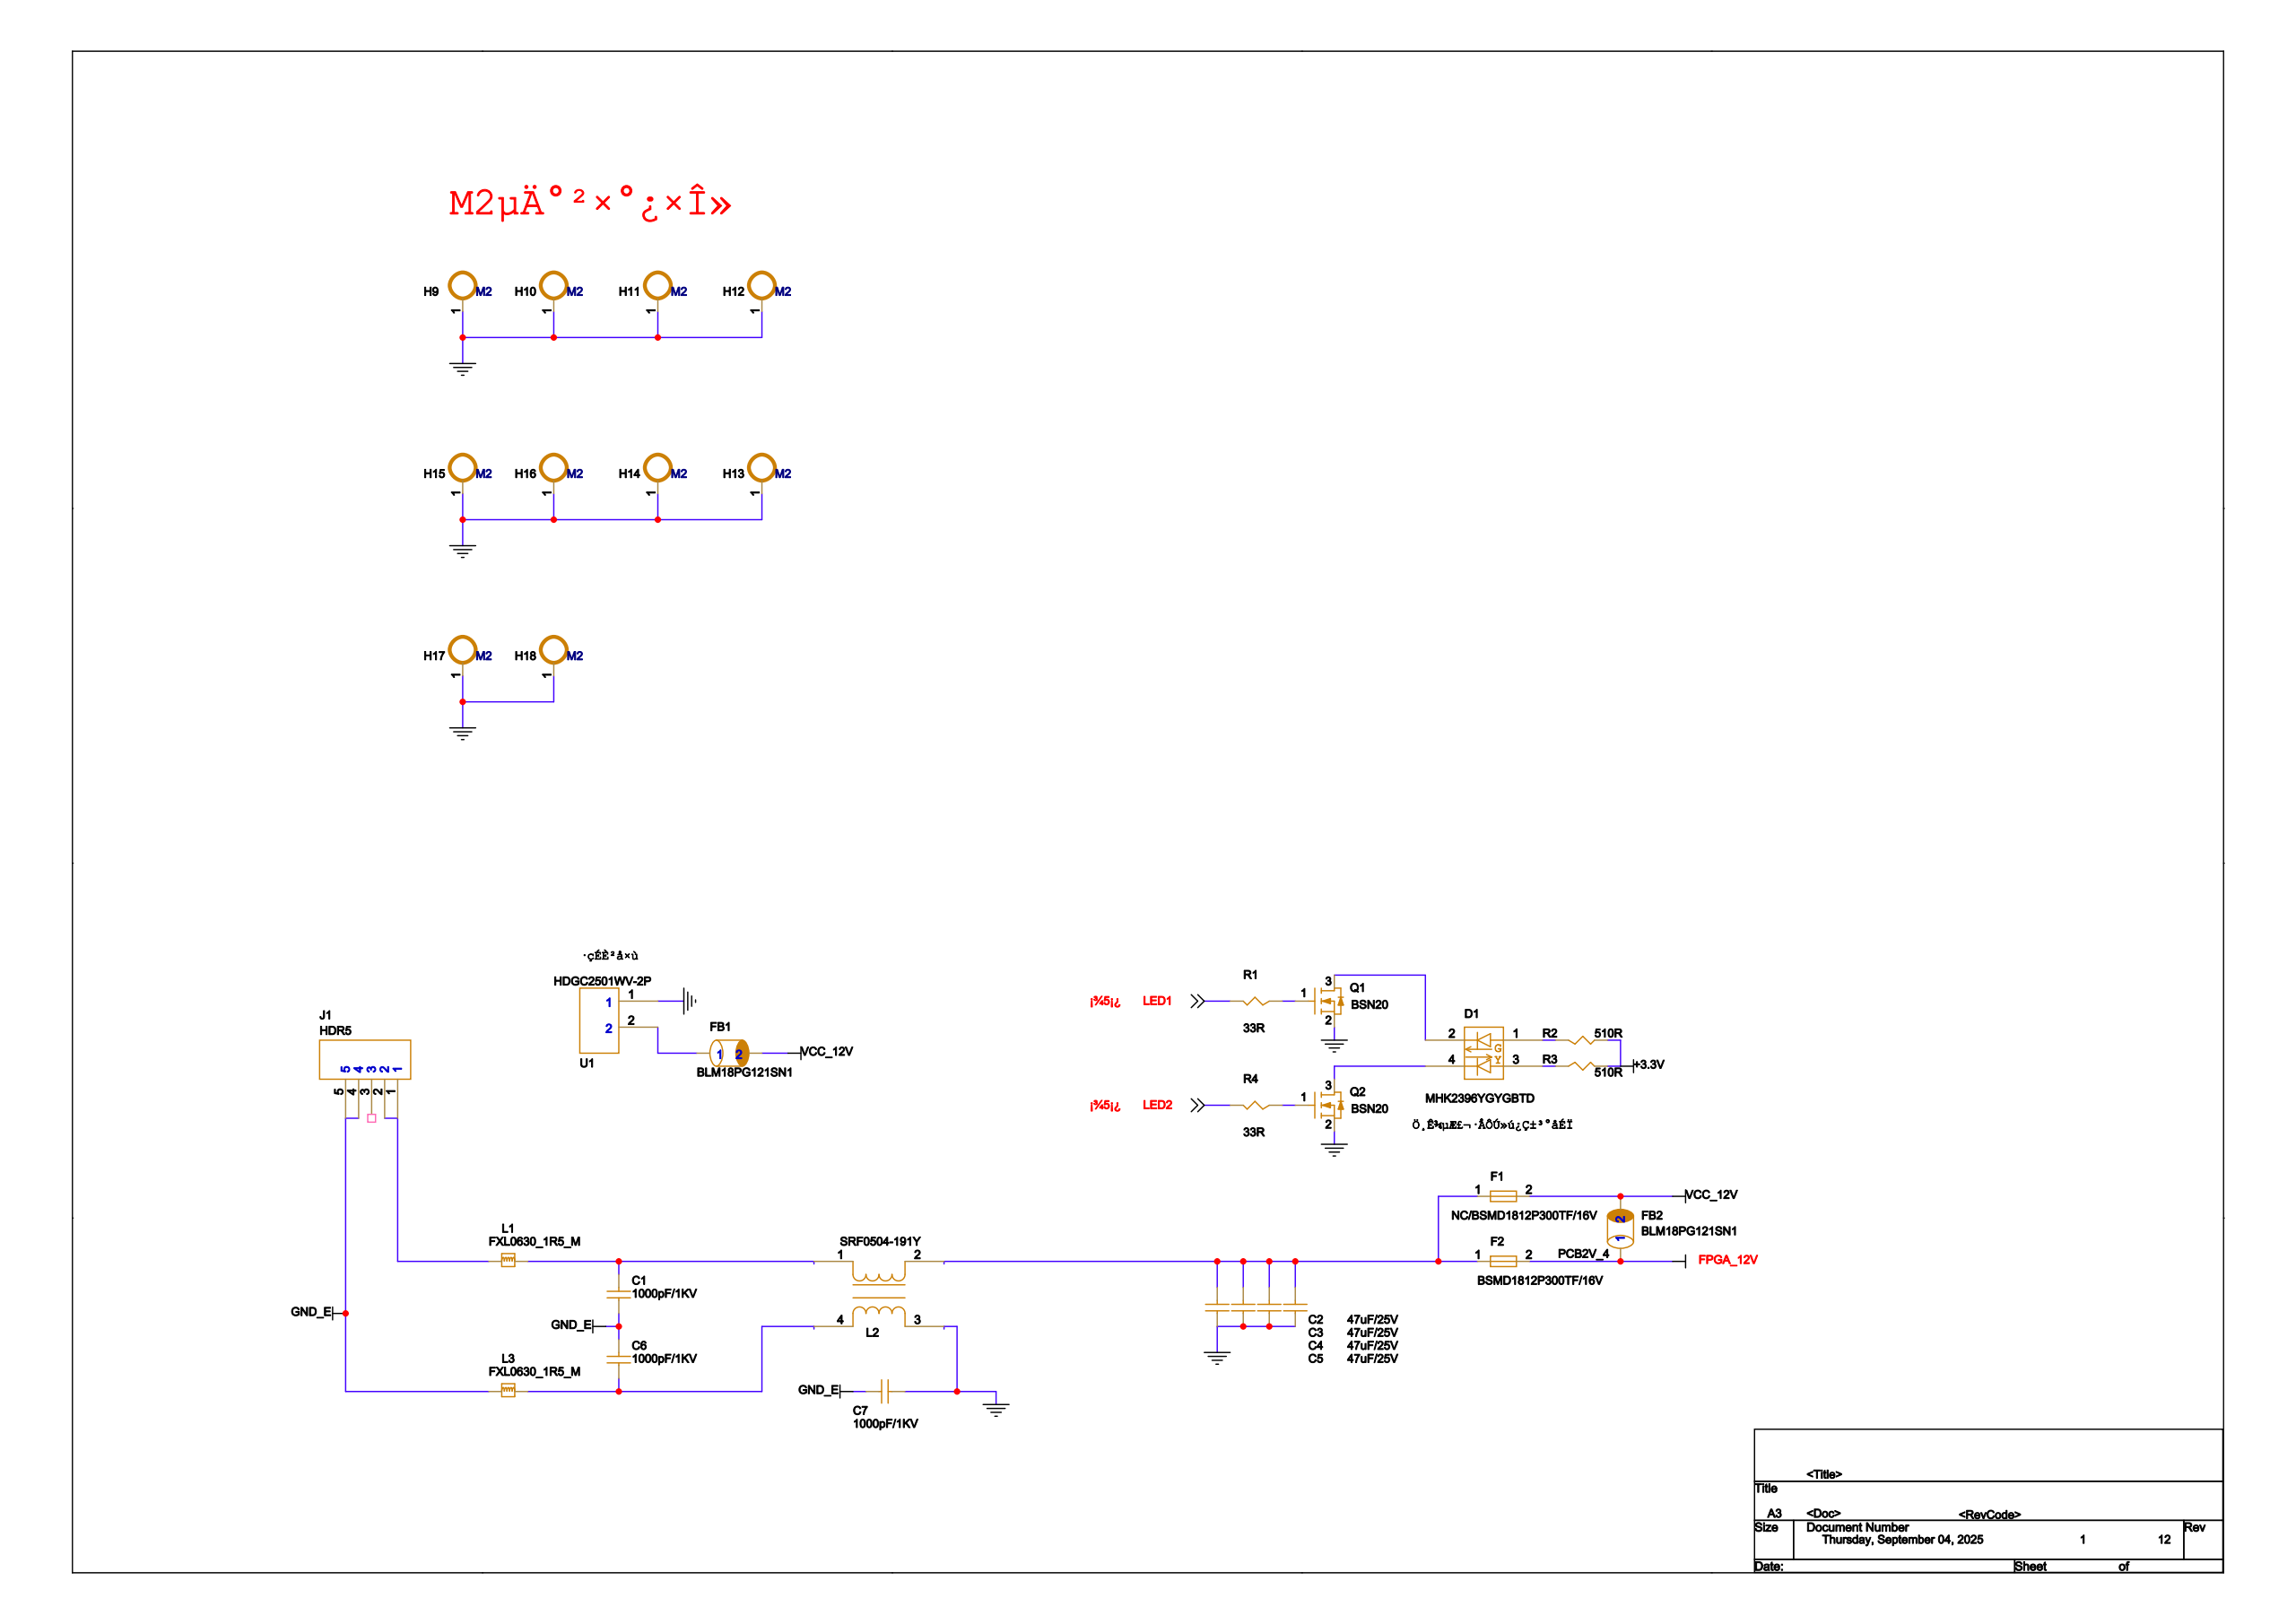Circuit board | Cadence Allegro | 528 parts | 530 nets | one sheet of the schematic
Parts on this sheet (reference | value | footprint):
C1 | 1000pF/1KV | C1206
C2 | 47uF/25V | C1206
C3 | 47uF/25V | C1206
C4 | 47uF/25V | C1206
C5 | 47uF/25V | C1206
C6 | 1000pF/1KV | C1206
C7 | 1000pF/1KV | C1206
D1 | MHK2396YGYGBTD | MHK2396YGYGBTD
F1 | NC/BSMD1812P300TF/16V | SMD1812
F2 | BSMD1812P300TF/16V | SMD1812
FB1 | BLM18PG121SN1 | 0603
FB2 | BLM18PG121SN1 | 0603
H9 | HOLE220D450 | GMPTH2_2R4_4
H10 | HOLE220D450 | GMPTH2_2R4_4
H11 | HOLE220D450 | GMPTH2_2R4_4
H12 | HOLE220D450 | GMPTH2_2R4_4
H13 | HOLE220D450 | GMPTH2_2R4_4
H14 | HOLE220D450 | GMPTH2_2R4_4
H15 | HOLE220D450 | GMPTH2_2R4_4
H16 | HOLE220D450 | GMPTH2_2R4_4
H17 | HOLE220D450 | GMPTH2_2R4_4
H18 | HOLE220D450 | GMPTH2_2R4_4
J1 | HDR5 | 2R54_5P
L1 | FXL0630_1R5_M | SMD_SMD_7X6_6
L2 | SRF0504-191Y | SFC-BNX027
L3 | FXL0630_1R5_M | SMD_SMD_7X6_6
Q1 | BSN20 | SOT-23
Q2 | BSN20 | SOT-23
R1 | 33R | R0402
R2 | 510R | R0402
R3 | 510R | R0402
R4 | 33R | R0402
U1 | HDGC2501WV-2P | CONN-TH_XH2_5-2P
Nets of these parts (net: part-pin ...):
GND: C2-1 C3-1 C4-1 C5-1 C7-2 H9-1 H10-1 H11-1 H12-1 H13-1 H14-1 H15-1 H16-1 H17-1 H18-1 L2-3 Q1-2 Q2-2 U1-1
VCC_12V: F1-2 FB1-2 FB2-2
+3.3V: R2-2 R3-2
GND_E: C1-1 C6-2 C7-1 J1-4 J1-5 L3-1
N17931932: C1-2 L1-2 L2-1
N17932110: C6-1 L2-4 L3-2
FPGA_12V: F2-2 FB2-1
N17931951: C2-2 C3-2 C4-2 C5-2 F1-1 F2-1 L2-2
N18543748: D1-1 R2-1
N18543690: D1-2 Q1-3
N18543770: D1-3 R3-1
N18543766: D1-4 Q2-3
N18090248: FB1-1 U1-2
N17931884: J1-1 J1-2 L1-1
N18543724: Q1-1 R1-1
N18543804: Q2-1 R4-1
LED1: R1-2
LED2: R4-2